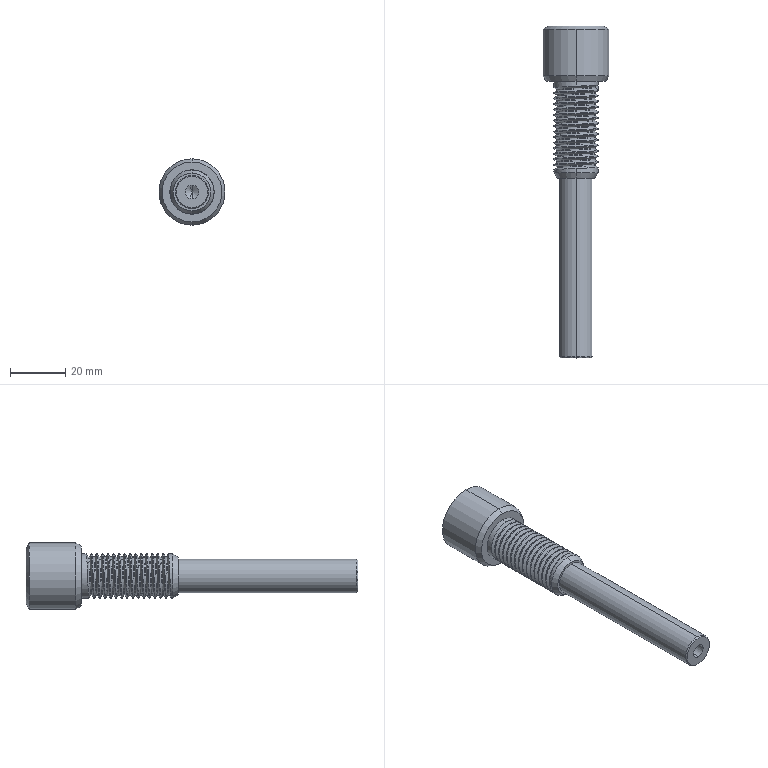Part | SolidWorks | features Chamfer 2, 3DProfileFeature 1, HoleWzd 1, Revolution 1, SweepThread 1 | 1 solid | 57 faces | box 24 x 120 x 24 mm | volume 22039 mm3 | cylinder 38 | cone 10 | plane 6 | spline 3 | commonest cylinder face diameters 16 x32 5 x2 12 x2 24 x2